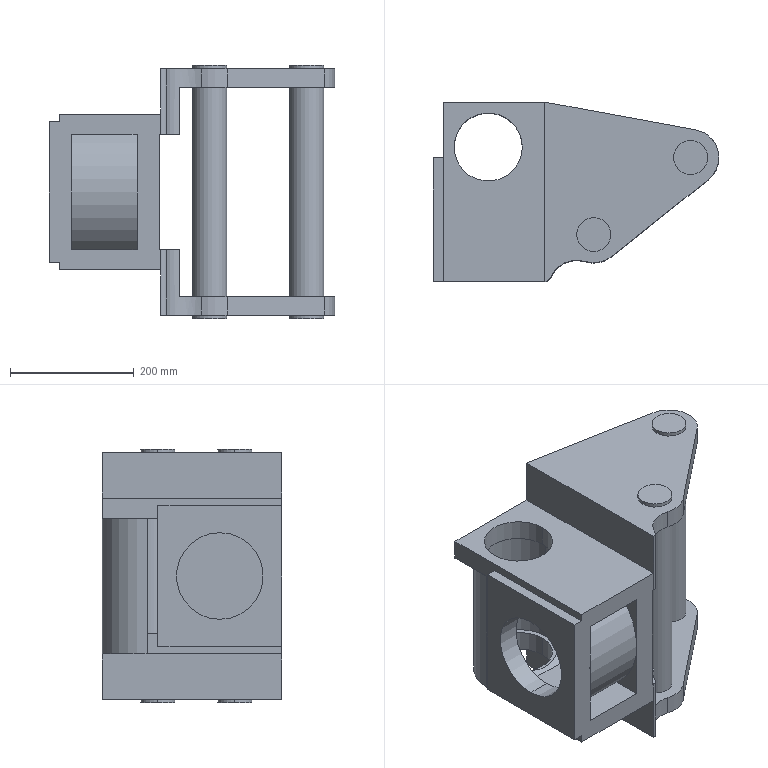Part | SolidWorks | features ICE 17, Extrusion 1, MirrorPattern 1 | 1 solid | 85 faces | box 461.6 x 289.885 x 410 mm | volume 11100203 mm3 | plane 47 | cylinder 38 | commonest cylinder face diameters 55 x12 91.2 x7 110 x4 140 x4 145 x3 198 x3